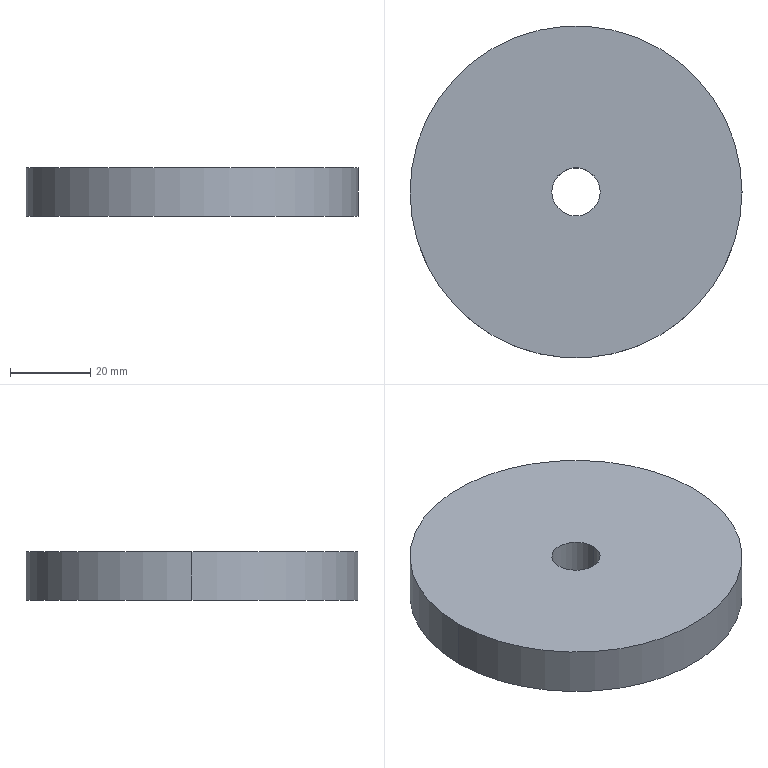Part | SolidWorks | features Extrusion 1 | 1 solid | 6 faces | box 82.5 x 82.5 x 12 mm | volume 62790 mm3 | cylinder 4 | plane 2 | commonest cylinder face diameters 12 x2 82.5 x2
STEP:
#1=CARTESIAN_POINT('',(-6.,0.,12.));
#2=VERTEX_POINT('',#1);
#3=CARTESIAN_POINT('',(6.,0.,12.));
#4=VERTEX_POINT('',#3);
#5=CARTESIAN_POINT('',(0.,0.,12.));
#6=DIRECTION('',(0.,0.,1.));
#7=DIRECTION('',(1.,0.,0.));
#8=AXIS2_PLACEMENT_3D('',#5,#6,#7);
#9=CIRCLE('',#8,6.);
#10=EDGE_CURVE('',#2,#4,#9,.T.);
#11=ORIENTED_EDGE('',*,*,#10,.T.);
#12=CARTESIAN_POINT('',(6.,0.,0.));
#13=VERTEX_POINT('',#12);
#14=CARTESIAN_POINT('',(6.,0.,12.));
#15=DIRECTION('',(0.,0.,-1.));
#16=VECTOR('',#15,1000.);
#17=LINE('',#14,#16);
#18=EDGE_CURVE('',#4,#13,#17,.T.);
#19=ORIENTED_EDGE('',*,*,#18,.T.);
#20=CARTESIAN_POINT('',(-6.,0.,0.));
#21=VERTEX_POINT('',#20);
#22=CARTESIAN_POINT('',(0.,0.,0.));
#23=DIRECTION('',(0.,0.,1.));
#24=DIRECTION('',(1.,0.,0.));
#25=AXIS2_PLACEMENT_3D('',#22,#23,#24);
#26=CIRCLE('',#25,6.);
#27=EDGE_CURVE('',#21,#13,#26,.T.);
#28=ORIENTED_EDGE('',*,*,#27,.F.);
#29=CARTESIAN_POINT('',(-6.,0.,12.));
#30=DIRECTION('',(0.,0.,-1.));
#31=VECTOR('',#30,1000.);
#32=LINE('',#29,#31);
#33=EDGE_CURVE('',#2,#21,#32,.T.);
#34=ORIENTED_EDGE('',*,*,#33,.F.);
#35=EDGE_LOOP('',(#11,#19,#28,#34));
#36=FACE_OUTER_BOUND('',#35,.T.);
#37=CARTESIAN_POINT('',(0.,0.,12.));
#38=DIRECTION('',(0.,0.,-1.));
#39=DIRECTION('',(-1.,0.,0.));
#40=AXIS2_PLACEMENT_3D('',#37,#38,#39);
#41=CYLINDRICAL_SURFACE('',#40,6.);
#42=ADVANCED_FACE('',(#36),#41,.F.);
#43=CARTESIAN_POINT('',(41.25,0.,12.));
#44=VERTEX_POINT('',#43);
#45=CARTESIAN_POINT('',(-41.25,0.,12.));
#46=VERTEX_POINT('',#45);
#47=CARTESIAN_POINT('',(0.,0.,12.));
#48=DIRECTION('',(0.,0.,1.));
#49=DIRECTION('',(1.,0.,0.));
#50=AXIS2_PLACEMENT_3D('',#47,#48,#49);
#51=CIRCLE('',#50,41.25);
#52=EDGE_CURVE('',#44,#46,#51,.T.);
#53=ORIENTED_EDGE('',*,*,#52,.F.);
#54=CARTESIAN_POINT('',(41.25,0.,0.));
#55=VERTEX_POINT('',#54);
#56=CARTESIAN_POINT('',(41.25,0.,12.));
#57=DIRECTION('',(0.,0.,-1.));
#58=VECTOR('',#57,1000.);
#59=LINE('',#56,#58);
#60=EDGE_CURVE('',#44,#55,#59,.T.);
#61=ORIENTED_EDGE('',*,*,#60,.T.);
#62=CARTESIAN_POINT('',(-41.25,0.,0.));
#63=VERTEX_POINT('',#62);
#64=CARTESIAN_POINT('',(0.,0.,0.));
#65=DIRECTION('',(0.,0.,1.));
#66=DIRECTION('',(1.,0.,0.));
#67=AXIS2_PLACEMENT_3D('',#64,#65,#66);
#68=CIRCLE('',#67,41.25);
#69=EDGE_CURVE('',#55,#63,#68,.T.);
#70=ORIENTED_EDGE('',*,*,#69,.T.);
#71=CARTESIAN_POINT('',(-41.25,0.,12.));
#72=DIRECTION('',(0.,0.,-1.));
#73=VECTOR('',#72,1000.);
#74=LINE('',#71,#73);
#75=EDGE_CURVE('',#46,#63,#74,.T.);
#76=ORIENTED_EDGE('',*,*,#75,.F.);
#77=EDGE_LOOP('',(#53,#61,#70,#76));
#78=FACE_OUTER_BOUND('',#77,.T.);
#79=CARTESIAN_POINT('',(0.,0.,12.));
#80=DIRECTION('',(0.,0.,-1.));
#81=DIRECTION('',(-1.,0.,0.));
#82=AXIS2_PLACEMENT_3D('',#79,#80,#81);
#83=CYLINDRICAL_SURFACE('',#82,41.25);
#84=ADVANCED_FACE('',(#78),#83,.T.);
#85=CARTESIAN_POINT('',(0.,0.,12.));
#86=DIRECTION('',(0.,0.,1.));
#87=DIRECTION('',(1.,0.,0.));
#88=AXIS2_PLACEMENT_3D('',#85,#86,#87);
#89=CIRCLE('',#88,41.25);
#90=EDGE_CURVE('',#46,#44,#89,.T.);
#91=ORIENTED_EDGE('',*,*,#90,.T.);
#92=ORIENTED_EDGE('',*,*,#52,.T.);
#93=EDGE_LOOP('',(#91,#92));
#94=FACE_OUTER_BOUND('',#93,.T.);
#95=ORIENTED_EDGE('',*,*,#10,.F.);
#96=CARTESIAN_POINT('',(0.,0.,12.));
#97=DIRECTION('',(0.,0.,1.));
#98=DIRECTION('',(1.,0.,0.));
#99=AXIS2_PLACEMENT_3D('',#96,#97,#98);
#100=CIRCLE('',#99,6.);
#101=EDGE_CURVE('',#4,#2,#100,.T.);
#102=ORIENTED_EDGE('',*,*,#101,.F.);
#103=EDGE_LOOP('',(#95,#102));
#104=FACE_BOUND('',#103,.T.);
#105=CARTESIAN_POINT('',(0.,0.,12.));
#106=DIRECTION('',(0.,0.,1.));
#107=DIRECTION('',(1.,0.,0.));
#108=AXIS2_PLACEMENT_3D('',#105,#106,#107);
#109=PLANE('',#108);
#110=ADVANCED_FACE('',(#94,#104),#109,.T.);
#111=CARTESIAN_POINT('',(0.,0.,0.));
#112=DIRECTION('',(0.,0.,1.));
#113=DIRECTION('',(1.,0.,0.));
#114=AXIS2_PLACEMENT_3D('',#111,#112,#113);
#115=CIRCLE('',#114,41.25);
#116=EDGE_CURVE('',#63,#55,#115,.T.);
#117=ORIENTED_EDGE('',*,*,#116,.F.);
#118=ORIENTED_EDGE('',*,*,#69,.F.);
#119=EDGE_LOOP('',(#117,#118));
#120=FACE_OUTER_BOUND('',#119,.T.);
#121=ORIENTED_EDGE('',*,*,#27,.T.);
#122=CARTESIAN_POINT('',(0.,0.,0.));
#123=DIRECTION('',(0.,0.,1.));
#124=DIRECTION('',(1.,0.,0.));
#125=AXIS2_PLACEMENT_3D('',#122,#123,#124);
#126=CIRCLE('',#125,6.);
#127=EDGE_CURVE('',#13,#21,#126,.T.);
#128=ORIENTED_EDGE('',*,*,#127,.T.);
#129=EDGE_LOOP('',(#121,#128));
#130=FACE_BOUND('',#129,.T.);
#131=CARTESIAN_POINT('',(0.,0.,0.));
#132=DIRECTION('',(0.,0.,1.));
#133=DIRECTION('',(1.,0.,0.));
#134=AXIS2_PLACEMENT_3D('',#131,#132,#133);
#135=PLANE('',#134);
#136=ADVANCED_FACE('',(#120,#130),#135,.F.);
#137=ORIENTED_EDGE('',*,*,#60,.F.);
#138=ORIENTED_EDGE('',*,*,#90,.F.);
#139=ORIENTED_EDGE('',*,*,#75,.T.);
#140=ORIENTED_EDGE('',*,*,#116,.T.);
#141=EDGE_LOOP('',(#137,#138,#139,#140));
#142=FACE_OUTER_BOUND('',#141,.T.);
#143=CARTESIAN_POINT('',(0.,0.,12.));
#144=DIRECTION('',(0.,0.,-1.));
#145=DIRECTION('',(-1.,0.,0.));
#146=AXIS2_PLACEMENT_3D('',#143,#144,#145);
#147=CYLINDRICAL_SURFACE('',#146,41.25);
#148=ADVANCED_FACE('',(#142),#147,.T.);
#149=ORIENTED_EDGE('',*,*,#18,.F.);
#150=ORIENTED_EDGE('',*,*,#101,.T.);
#151=ORIENTED_EDGE('',*,*,#33,.T.);
#152=ORIENTED_EDGE('',*,*,#127,.F.);
#153=EDGE_LOOP('',(#149,#150,#151,#152));
#154=FACE_OUTER_BOUND('',#153,.T.);
#155=CARTESIAN_POINT('',(0.,0.,12.));
#156=DIRECTION('',(0.,0.,-1.));
#157=DIRECTION('',(-1.,0.,0.));
#158=AXIS2_PLACEMENT_3D('',#155,#156,#157);
#159=CYLINDRICAL_SURFACE('',#158,6.);
#160=ADVANCED_FACE('',(#154),#159,.F.);
#161=CLOSED_SHELL('',(#42,#84,#110,#136,#148,#160));
#162=MANIFOLD_SOLID_BREP('',#161);
#163=CARTESIAN_POINT('',(0.,0.,0.));
#164=DIRECTION('',(0.,0.,1.));
#165=DIRECTION('',(1.,0.,0.));
#166=AXIS2_PLACEMENT_3D('',#163,#164,#165);
#167=(LENGTH_UNIT()NAMED_UNIT(*)SI_UNIT(.MILLI.,.METRE.));
#168=UNCERTAINTY_MEASURE_WITH_UNIT(LENGTH_MEASURE(0.00001),#167,'','');
#169=(NAMED_UNIT(*)PLANE_ANGLE_UNIT()SI_UNIT($,.RADIAN.));
#170=(NAMED_UNIT(*)SI_UNIT($,.STERADIAN.)SOLID_ANGLE_UNIT());
#171=(GEOMETRIC_REPRESENTATION_CONTEXT(3)GLOBAL_UNCERTAINTY_ASSIGNED_CONTEXT((#168))GLOBAL_UNIT_ASSIGNED_CONTEXT((#167,#169,#170))REPRESENTATION_CONTEXT('',''));
#172=ADVANCED_BREP_SHAPE_REPRESENTATION('',(#162,#166),#171);